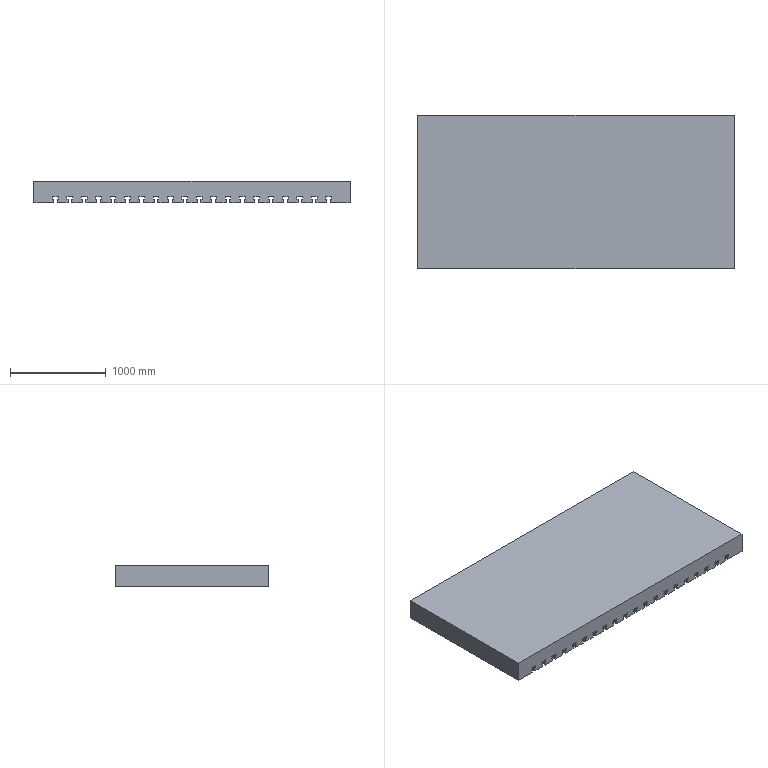Part | NX | features solid 2 | 1 solid | 202 faces | box 3300 x 1600 x 220 mm | volume 1071834762 mm3 | plane 198 | cylinder 4 | commonest cylinder face diameters 69 x4